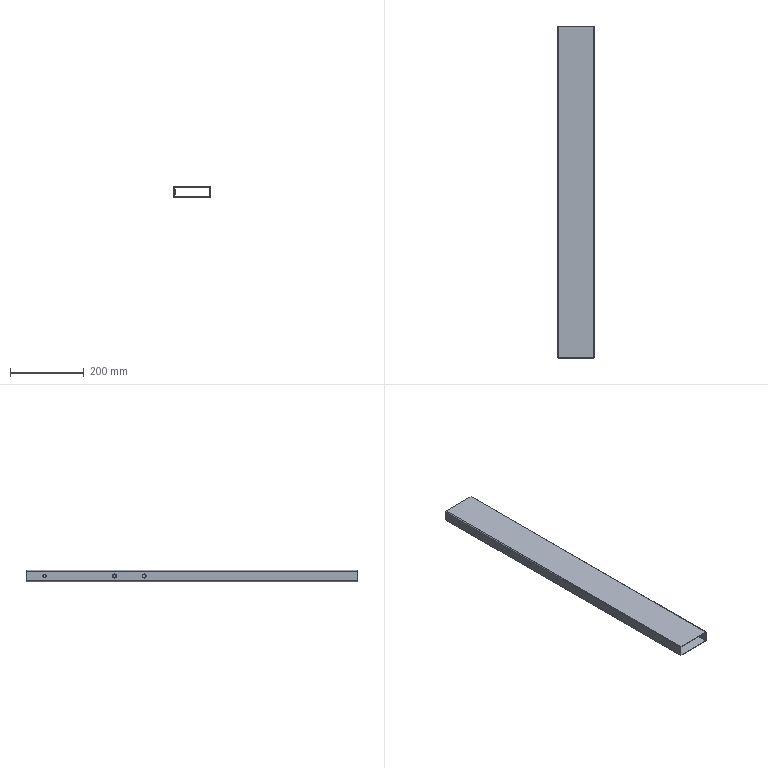Part | STEP file | 7470201L | 1 solid | 29 faces | box 100 x 900 x 30 mm | volume 338694 mm3 | cylinder 15 | plane 12 | torus 2 | commonest cylinder face diameters 2 x4 5 x4 9 x3 8 x2 11 x2